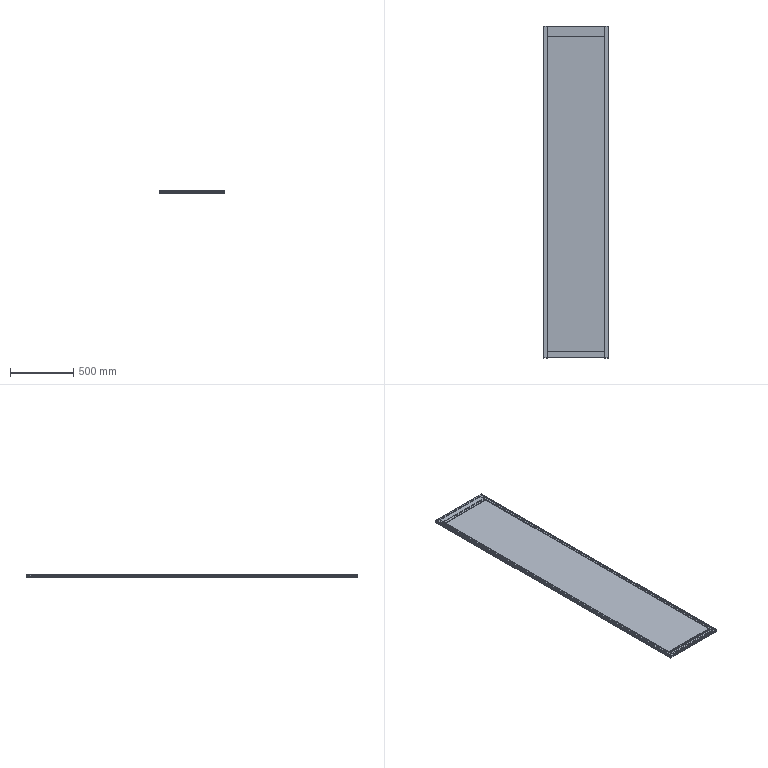Part | 5 solids | 330 faces | box 510 x 2616 x 20.2 mm | volume 13203420 mm3 | cylinder 180 | plane 150 | commonest cylinder face diameters 0.6 x48 13 x48 0.4 x27 1 x21 9 x16 7.2 x12